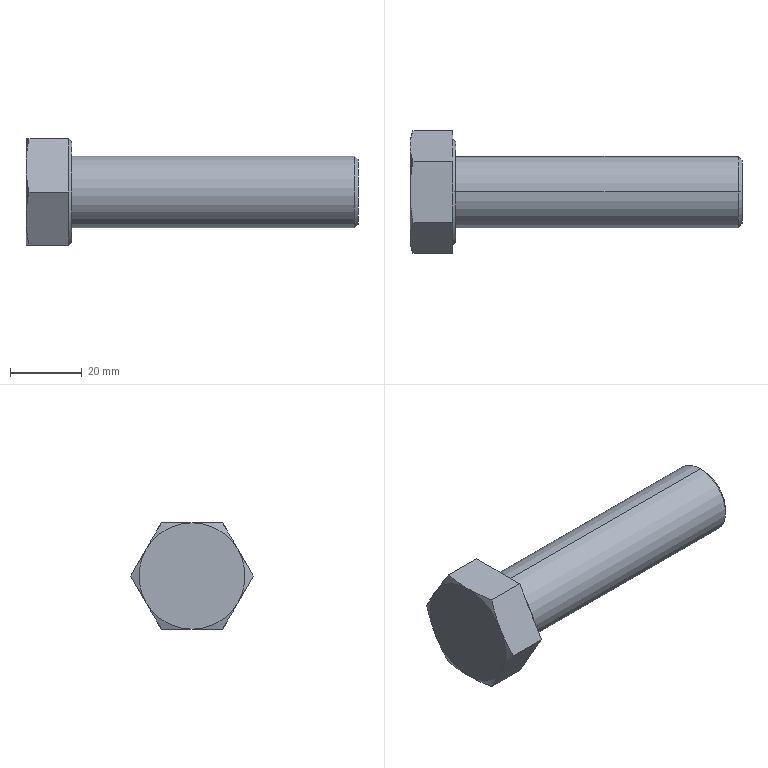Part | SolidWorks | features RevCut 3, Boss 1, Chamfer 1, Extrusion 1, Fillet 1, LPattern 1 | 1 solid | 27 faces | box 92.715 x 34.26 x 29.67 mm | volume 34696 mm3 | plane 15 | cone 10 | cylinder 2 | commonest cylinder face diameters 20 x2
STEP:
#1=CARTESIAN_POINT('',(92.715,0.,-9.));
#2=VERTEX_POINT('',#1);
#3=CARTESIAN_POINT('',(92.715,0.,9.));
#4=VERTEX_POINT('',#3);
#5=CARTESIAN_POINT('',(92.715,0.,0.));
#6=DIRECTION('',(1.,0.,0.));
#7=DIRECTION('',(0.,0.,-1.));
#8=AXIS2_PLACEMENT_3D('',#5,#6,#7);
#9=CIRCLE('',#8,9.);
#10=EDGE_CURVE('',#2,#4,#9,.T.);
#11=ORIENTED_EDGE('',*,*,#10,.F.);
#12=CARTESIAN_POINT('',(91.715,0.,-10.));
#13=VERTEX_POINT('',#12);
#14=CARTESIAN_POINT('',(92.715,0.,-9.));
#15=DIRECTION('',(-0.7071,0.,-0.7071));
#16=VECTOR('',#15,1000.);
#17=LINE('',#14,#16);
#18=EDGE_CURVE('',#2,#13,#17,.T.);
#19=ORIENTED_EDGE('',*,*,#18,.T.);
#20=CARTESIAN_POINT('',(91.715,0.,10.));
#21=VERTEX_POINT('',#20);
#22=CARTESIAN_POINT('',(91.715,0.,0.));
#23=DIRECTION('',(-1.,0.,0.));
#24=DIRECTION('',(0.,0.,-1.));
#25=AXIS2_PLACEMENT_3D('',#22,#23,#24);
#26=CIRCLE('',#25,10.);
#27=EDGE_CURVE('',#21,#13,#26,.T.);
#28=ORIENTED_EDGE('',*,*,#27,.F.);
#29=CARTESIAN_POINT('',(92.715,0.,9.));
#30=DIRECTION('',(-0.7071,0.,0.7071));
#31=VECTOR('',#30,1000.);
#32=LINE('',#29,#31);
#33=EDGE_CURVE('',#4,#21,#32,.T.);
#34=ORIENTED_EDGE('',*,*,#33,.F.);
#35=EDGE_LOOP('',(#11,#19,#28,#34));
#36=FACE_OUTER_BOUND('',#35,.T.);
#37=CARTESIAN_POINT('',(92.715,0.,0.));
#38=DIRECTION('',(-1.,0.,0.));
#39=DIRECTION('',(0.,0.,1.));
#40=AXIS2_PLACEMENT_3D('',#37,#38,#39);
#41=CONICAL_SURFACE('',#40,9.,0.7854);
#42=ADVANCED_FACE('',(#36),#41,.T.);
#43=ORIENTED_EDGE('',*,*,#27,.T.);
#44=CARTESIAN_POINT('',(12.715,0.,-10.));
#45=VERTEX_POINT('',#44);
#46=CARTESIAN_POINT('',(92.715,0.,-10.));
#47=DIRECTION('',(-1.,0.,0.));
#48=VECTOR('',#47,1000.);
#49=LINE('',#46,#48);
#50=EDGE_CURVE('',#13,#45,#49,.T.);
#51=ORIENTED_EDGE('',*,*,#50,.T.);
#52=CARTESIAN_POINT('',(12.715,0.,10.));
#53=VERTEX_POINT('',#52);
#54=CARTESIAN_POINT('',(12.715,0.,0.));
#55=DIRECTION('',(1.,0.,0.));
#56=DIRECTION('',(0.,0.,-1.));
#57=AXIS2_PLACEMENT_3D('',#54,#55,#56);
#58=CIRCLE('',#57,10.);
#59=EDGE_CURVE('',#45,#53,#58,.T.);
#60=ORIENTED_EDGE('',*,*,#59,.T.);
#61=CARTESIAN_POINT('',(92.715,0.,10.));
#62=DIRECTION('',(-1.,0.,0.));
#63=VECTOR('',#62,1000.);
#64=LINE('',#61,#63);
#65=EDGE_CURVE('',#21,#53,#64,.T.);
#66=ORIENTED_EDGE('',*,*,#65,.F.);
#67=EDGE_LOOP('',(#43,#51,#60,#66));
#68=FACE_OUTER_BOUND('',#67,.T.);
#69=CARTESIAN_POINT('',(92.715,0.,0.));
#70=DIRECTION('',(-1.,0.,0.));
#71=DIRECTION('',(0.,0.,1.));
#72=AXIS2_PLACEMENT_3D('',#69,#70,#71);
#73=CYLINDRICAL_SURFACE('',#72,10.);
#74=ADVANCED_FACE('',(#68),#73,.T.);
#75=CARTESIAN_POINT('',(12.715,0.,14.095));
#76=VERTEX_POINT('',#75);
#77=CARTESIAN_POINT('',(12.715,0.,-14.095));
#78=VERTEX_POINT('',#77);
#79=CARTESIAN_POINT('',(12.715,0.,0.));
#80=DIRECTION('',(-1.,0.,0.));
#81=DIRECTION('',(0.,0.,1.));
#82=AXIS2_PLACEMENT_3D('',#79,#80,#81);
#83=CIRCLE('',#82,14.095);
#84=EDGE_CURVE('',#76,#78,#83,.T.);
#85=ORIENTED_EDGE('',*,*,#84,.T.);
#86=CARTESIAN_POINT('',(11.975,0.,-14.835));
#87=VERTEX_POINT('',#86);
#88=CARTESIAN_POINT('',(11.915,0.,-14.895));
#89=DIRECTION('',(-0.7071,0.,-0.7071));
#90=VECTOR('',#89,1000.);
#91=LINE('',#88,#90);
#92=EDGE_CURVE('',#78,#87,#91,.T.);
#93=ORIENTED_EDGE('',*,*,#92,.T.);
#94=CARTESIAN_POINT('',(11.915,1.336,-14.835));
#95=VERTEX_POINT('',#94);
#96=CARTESIAN_POINT('',(11.975,0.,-14.835));
#97=CARTESIAN_POINT('',(11.975,0.4454,-14.835));
#98=CARTESIAN_POINT('',(11.955,0.8906,-14.835));
#99=CARTESIAN_POINT('',(11.915,1.336,-14.835));
#100=B_SPLINE_CURVE_WITH_KNOTS('',3,(#96,#97,#98,#99),.UNSPECIFIED.,.F.,.F.,(4,4),(0.008338,0.009669),.UNSPECIFIED.);
#101=EDGE_CURVE('',#87,#95,#100,.T.);
#102=ORIENTED_EDGE('',*,*,#101,.T.);
#103=CARTESIAN_POINT('',(11.915,12.18,-8.574));
#104=VERTEX_POINT('',#103);
#105=CARTESIAN_POINT('',(11.915,0.,0.));
#106=DIRECTION('',(-1.,0.,0.));
#107=DIRECTION('',(0.,0.,1.));
#108=AXIS2_PLACEMENT_3D('',#105,#106,#107);
#109=CIRCLE('',#108,14.895);
#110=EDGE_CURVE('',#104,#95,#109,.T.);
#111=ORIENTED_EDGE('',*,*,#110,.F.);
#112=CARTESIAN_POINT('',(11.915,13.515,-6.261));
#113=VERTEX_POINT('',#112);
#114=CARTESIAN_POINT('',(11.915,12.18,-8.574));
#115=CARTESIAN_POINT('',(11.995,12.625,-7.803));
#116=CARTESIAN_POINT('',(11.995,13.07,-7.032));
#117=CARTESIAN_POINT('',(11.915,13.515,-6.261));
#118=B_SPLINE_CURVE_WITH_KNOTS('',3,(#114,#115,#116,#117),.UNSPECIFIED.,.F.,.F.,(4,4),(0.000002229,0.002673),.UNSPECIFIED.);
#119=EDGE_CURVE('',#104,#113,#118,.T.);
#120=ORIENTED_EDGE('',*,*,#119,.T.);
#121=CARTESIAN_POINT('',(11.915,13.515,6.261));
#122=VERTEX_POINT('',#121);
#123=CARTESIAN_POINT('',(11.915,0.,0.));
#124=DIRECTION('',(-1.,0.,0.));
#125=DIRECTION('',(0.,0.,1.));
#126=AXIS2_PLACEMENT_3D('',#123,#124,#125);
#127=CIRCLE('',#126,14.895);
#128=EDGE_CURVE('',#122,#113,#127,.T.);
#129=ORIENTED_EDGE('',*,*,#128,.F.);
#130=CARTESIAN_POINT('',(11.915,12.18,8.574));
#131=VERTEX_POINT('',#130);
#132=CARTESIAN_POINT('',(11.915,13.515,6.261));
#133=CARTESIAN_POINT('',(11.995,13.07,7.032));
#134=CARTESIAN_POINT('',(11.995,12.625,7.803));
#135=CARTESIAN_POINT('',(11.915,12.18,8.574));
#136=B_SPLINE_CURVE_WITH_KNOTS('',3,(#132,#133,#134,#135),.UNSPECIFIED.,.F.,.F.,(4,4),(0.000002229,0.002673),.UNSPECIFIED.);
#137=EDGE_CURVE('',#122,#131,#136,.T.);
#138=ORIENTED_EDGE('',*,*,#137,.T.);
#139=CARTESIAN_POINT('',(11.915,1.336,14.835));
#140=VERTEX_POINT('',#139);
#141=CARTESIAN_POINT('',(11.915,0.,0.));
#142=DIRECTION('',(-1.,0.,0.));
#143=DIRECTION('',(0.,0.,1.));
#144=AXIS2_PLACEMENT_3D('',#141,#142,#143);
#145=CIRCLE('',#144,14.895);
#146=EDGE_CURVE('',#140,#131,#145,.T.);
#147=ORIENTED_EDGE('',*,*,#146,.F.);
#148=CARTESIAN_POINT('',(11.975,0.,14.835));
#149=VERTEX_POINT('',#148);
#150=CARTESIAN_POINT('',(11.915,1.336,14.835));
#151=CARTESIAN_POINT('',(11.955,0.8906,14.835));
#152=CARTESIAN_POINT('',(11.975,0.4454,14.835));
#153=CARTESIAN_POINT('',(11.975,0.,14.835));
#154=B_SPLINE_CURVE_WITH_KNOTS('',3,(#150,#151,#152,#153),.UNSPECIFIED.,.F.,.F.,(4,4),(0.007682,0.009012),.UNSPECIFIED.);
#155=EDGE_CURVE('',#140,#149,#154,.T.);
#156=ORIENTED_EDGE('',*,*,#155,.T.);
#157=CARTESIAN_POINT('',(11.915,0.,14.895));
#158=DIRECTION('',(-0.7071,0.,0.7071));
#159=VECTOR('',#158,1000.);
#160=LINE('',#157,#159);
#161=EDGE_CURVE('',#76,#149,#160,.T.);
#162=ORIENTED_EDGE('',*,*,#161,.F.);
#163=EDGE_LOOP('',(#85,#93,#102,#111,#120,#129,#138,#147,#156,#162));
#164=FACE_OUTER_BOUND('',#163,.T.);
#165=CARTESIAN_POINT('',(11.915,0.,0.));
#166=DIRECTION('',(-1.,0.,0.));
#167=DIRECTION('',(0.,0.,1.));
#168=AXIS2_PLACEMENT_3D('',#165,#166,#167);
#169=CONICAL_SURFACE('',#168,14.895,0.7854);
#170=ADVANCED_FACE('',(#164),#169,.T.);
#171=ORIENTED_EDGE('',*,*,#84,.F.);
#172=CARTESIAN_POINT('',(12.715,0.,0.));
#173=DIRECTION('',(-1.,0.,0.));
#174=DIRECTION('',(0.,0.,1.));
#175=AXIS2_PLACEMENT_3D('',#172,#173,#174);
#176=CIRCLE('',#175,14.095);
#177=EDGE_CURVE('',#78,#76,#176,.T.);
#178=ORIENTED_EDGE('',*,*,#177,.F.);
#179=EDGE_LOOP('',(#171,#178));
#180=FACE_OUTER_BOUND('',#179,.T.);
#181=CARTESIAN_POINT('',(12.715,0.,0.));
#182=DIRECTION('',(1.,0.,0.));
#183=DIRECTION('',(0.,0.,-1.));
#184=AXIS2_PLACEMENT_3D('',#181,#182,#183);
#185=CIRCLE('',#184,10.);
#186=EDGE_CURVE('',#53,#45,#185,.T.);
#187=ORIENTED_EDGE('',*,*,#186,.F.);
#188=ORIENTED_EDGE('',*,*,#59,.F.);
#189=EDGE_LOOP('',(#187,#188));
#190=FACE_BOUND('',#189,.T.);
#191=CARTESIAN_POINT('',(12.715,-8.565,-14.835));
#192=DIRECTION('',(1.,0.,0.));
#193=DIRECTION('',(0.,0.,-1.));
#194=AXIS2_PLACEMENT_3D('',#191,#192,#193);
#195=PLANE('',#194);
#196=ADVANCED_FACE('',(#180,#190),#195,.T.);
#197=CARTESIAN_POINT('',(0.8353,-8.565,-14.835));
#198=VERTEX_POINT('',#197);
#199=CARTESIAN_POINT('',(0.,-12.847,-7.417));
#200=VERTEX_POINT('',#199);
#201=CARTESIAN_POINT('',(0.8353,-8.565,-14.835));
#202=CARTESIAN_POINT('',(0.5755,-9.279,-13.599));
#203=CARTESIAN_POINT('',(0.3646,-9.992,-12.363));
#204=CARTESIAN_POINT('',(0.07638,-11.42,-9.89));
#205=CARTESIAN_POINT('',(0.,-12.134,-8.654));
#206=CARTESIAN_POINT('',(0.,-12.847,-7.417));
#207=B_SPLINE_CURVE_WITH_KNOTS('',3,(#201,#202,#203,#204,#205,#206),.UNSPECIFIED.,.F.,.F.,(4,2,4),(0.000000231,0.004283,0.008565),.UNSPECIFIED.);
#208=EDGE_CURVE('',#198,#200,#207,.T.);
#209=ORIENTED_EDGE('',*,*,#208,.F.);
#210=CARTESIAN_POINT('',(11.915,-8.565,-14.835));
#211=VERTEX_POINT('',#210);
#212=CARTESIAN_POINT('',(12.715,-8.565,-14.835));
#213=DIRECTION('',(-1.,0.,0.));
#214=VECTOR('',#213,1000.);
#215=LINE('',#212,#214);
#216=EDGE_CURVE('',#211,#198,#215,.T.);
#217=ORIENTED_EDGE('',*,*,#216,.F.);
#218=CARTESIAN_POINT('',(11.915,-12.18,-8.574));
#219=VERTEX_POINT('',#218);
#220=CARTESIAN_POINT('',(11.915,-17.13,0.));
#221=DIRECTION('',(0.,0.5,-0.866));
#222=VECTOR('',#221,1000.);
#223=LINE('',#220,#222);
#224=EDGE_CURVE('',#219,#211,#223,.T.);
#225=ORIENTED_EDGE('',*,*,#224,.F.);
#226=CARTESIAN_POINT('',(11.915,-13.515,-6.261));
#227=VERTEX_POINT('',#226);
#228=CARTESIAN_POINT('',(11.915,-13.515,-6.261));
#229=CARTESIAN_POINT('',(11.995,-13.07,-7.032));
#230=CARTESIAN_POINT('',(11.995,-12.625,-7.803));
#231=CARTESIAN_POINT('',(11.915,-12.18,-8.574));
#232=B_SPLINE_CURVE_WITH_KNOTS('',3,(#228,#229,#230,#231),.UNSPECIFIED.,.F.,.F.,(4,4),(0.000002229,0.002673),.UNSPECIFIED.);
#233=EDGE_CURVE('',#227,#219,#232,.T.);
#234=ORIENTED_EDGE('',*,*,#233,.F.);
#235=CARTESIAN_POINT('',(11.915,-17.13,0.));
#236=VERTEX_POINT('',#235);
#237=CARTESIAN_POINT('',(11.915,-17.13,0.));
#238=DIRECTION('',(0.,0.5,-0.866));
#239=VECTOR('',#238,1000.);
#240=LINE('',#237,#239);
#241=EDGE_CURVE('',#236,#227,#240,.T.);
#242=ORIENTED_EDGE('',*,*,#241,.F.);
#243=CARTESIAN_POINT('',(0.8353,-17.13,0.));
#244=VERTEX_POINT('',#243);
#245=CARTESIAN_POINT('',(12.715,-17.13,0.));
#246=DIRECTION('',(-1.,0.,0.));
#247=VECTOR('',#246,1000.);
#248=LINE('',#245,#247);
#249=EDGE_CURVE('',#236,#244,#248,.T.);
#250=ORIENTED_EDGE('',*,*,#249,.T.);
#251=CARTESIAN_POINT('',(0.,-12.847,-7.417));
#252=CARTESIAN_POINT('',(0.,-13.561,-6.181));
#253=CARTESIAN_POINT('',(0.07638,-14.275,-4.945));
#254=CARTESIAN_POINT('',(0.3646,-15.702,-2.472));
#255=CARTESIAN_POINT('',(0.5755,-16.416,-1.236));
#256=CARTESIAN_POINT('',(0.8353,-17.13,0.));
#257=B_SPLINE_CURVE_WITH_KNOTS('',3,(#251,#252,#253,#254,#255,#256),.UNSPECIFIED.,.F.,.F.,(4,2,4),(0.008565,0.01285,0.01713),.UNSPECIFIED.);
#258=EDGE_CURVE('',#200,#244,#257,.T.);
#259=ORIENTED_EDGE('',*,*,#258,.F.);
#260=EDGE_LOOP('',(#209,#217,#225,#234,#242,#250,#259));
#261=FACE_OUTER_BOUND('',#260,.T.);
#262=CARTESIAN_POINT('',(12.715,-17.13,0.));
#263=DIRECTION('',(0.,0.866,0.5));
#264=DIRECTION('',(0.,-0.5,0.866));
#265=AXIS2_PLACEMENT_3D('',#262,#263,#264);
#266=PLANE('',#265);
#267=ADVANCED_FACE('',(#261),#266,.F.);
#268=CARTESIAN_POINT('',(0.8353,8.565,-14.835));
#269=VERTEX_POINT('',#268);
#270=CARTESIAN_POINT('',(0.,0.,-14.835));
#271=VERTEX_POINT('',#270);
#272=CARTESIAN_POINT('',(0.8353,8.565,-14.835));
#273=CARTESIAN_POINT('',(0.5762,7.141,-14.835));
#274=CARTESIAN_POINT('',(0.3651,5.714,-14.835));
#275=CARTESIAN_POINT('',(0.07668,2.859,-14.835));
#276=CARTESIAN_POINT('',(0.,1.43,-14.835));
#277=CARTESIAN_POINT('',(0.,0.,-14.835));
#278=B_SPLINE_CURVE_WITH_KNOTS('',3,(#272,#273,#274,#275,#276,#277),.UNSPECIFIED.,.F.,.F.,(4,2,4),(0.03088,0.0352,0.03952),.UNSPECIFIED.);
#279=EDGE_CURVE('',#269,#271,#278,.T.);
#280=ORIENTED_EDGE('',*,*,#279,.F.);
#281=CARTESIAN_POINT('',(11.915,8.565,-14.835));
#282=VERTEX_POINT('',#281);
#283=CARTESIAN_POINT('',(12.715,8.565,-14.835));
#284=DIRECTION('',(-1.,0.,0.));
#285=VECTOR('',#284,1000.);
#286=LINE('',#283,#285);
#287=EDGE_CURVE('',#282,#269,#286,.T.);
#288=ORIENTED_EDGE('',*,*,#287,.F.);
#289=CARTESIAN_POINT('',(11.915,-8.565,-14.835));
#290=DIRECTION('',(0.,1.,0.));
#291=VECTOR('',#290,1000.);
#292=LINE('',#289,#291);
#293=EDGE_CURVE('',#95,#282,#292,.T.);
#294=ORIENTED_EDGE('',*,*,#293,.F.);
#295=ORIENTED_EDGE('',*,*,#101,.F.);
#296=CARTESIAN_POINT('',(11.915,-1.336,-14.835));
#297=VERTEX_POINT('',#296);
#298=CARTESIAN_POINT('',(11.915,-1.336,-14.835));
#299=CARTESIAN_POINT('',(11.955,-0.8902,-14.835));
#300=CARTESIAN_POINT('',(11.975,-0.445,-14.835));
#301=CARTESIAN_POINT('',(11.975,0.,-14.835));
#302=B_SPLINE_CURVE_WITH_KNOTS('',3,(#298,#299,#300,#301),.UNSPECIFIED.,.F.,.F.,(4,4),(0.007008,0.008338),.UNSPECIFIED.);
#303=EDGE_CURVE('',#297,#87,#302,.T.);
#304=ORIENTED_EDGE('',*,*,#303,.F.);
#305=CARTESIAN_POINT('',(11.915,-8.565,-14.835));
#306=DIRECTION('',(0.,1.,0.));
#307=VECTOR('',#306,1000.);
#308=LINE('',#305,#307);
#309=EDGE_CURVE('',#211,#297,#308,.T.);
#310=ORIENTED_EDGE('',*,*,#309,.F.);
#311=ORIENTED_EDGE('',*,*,#216,.T.);
#312=CARTESIAN_POINT('',(0.,0.,-14.835));
#313=CARTESIAN_POINT('',(0.,-1.426,-14.835));
#314=CARTESIAN_POINT('',(0.07627,-2.854,-14.835));
#315=CARTESIAN_POINT('',(0.3649,-5.713,-14.835));
#316=CARTESIAN_POINT('',(0.5772,-7.147,-14.835));
#317=CARTESIAN_POINT('',(0.8353,-8.565,-14.835));
#318=B_SPLINE_CURVE_WITH_KNOTS('',3,(#312,#313,#314,#315,#316,#317),.UNSPECIFIED.,.F.,.F.,(4,2,4),(0.03952,0.04383,0.04813),.UNSPECIFIED.);
#319=EDGE_CURVE('',#271,#198,#318,.T.);
#320=ORIENTED_EDGE('',*,*,#319,.F.);
#321=EDGE_LOOP('',(#280,#288,#294,#295,#304,#310,#311,#320));
#322=FACE_OUTER_BOUND('',#321,.T.);
#323=CARTESIAN_POINT('',(12.715,-8.565,-14.835));
#324=DIRECTION('',(0.,0.,1.));
#325=DIRECTION('',(1.,0.,0.));
#326=AXIS2_PLACEMENT_3D('',#323,#324,#325);
#327=PLANE('',#326);
#328=ADVANCED_FACE('',(#322),#327,.F.);
#329=CARTESIAN_POINT('',(0.8353,17.13,0.));
#330=VERTEX_POINT('',#329);
#331=CARTESIAN_POINT('',(0.,12.847,-7.418));
#332=VERTEX_POINT('',#331);
#333=CARTESIAN_POINT('',(0.8353,17.13,0.));
#334=CARTESIAN_POINT('',(0.5755,16.416,-1.236));
#335=CARTESIAN_POINT('',(0.3646,15.702,-2.472));
#336=CARTESIAN_POINT('',(0.07638,14.275,-4.945));
#337=CARTESIAN_POINT('',(0.,13.561,-6.181));
#338=CARTESIAN_POINT('',(0.,12.847,-7.418));
#339=B_SPLINE_CURVE_WITH_KNOTS('',3,(#333,#334,#335,#336,#337,#338),.UNSPECIFIED.,.F.,.F.,(4,2,4),(0.000000231,0.004283,0.008565),.UNSPECIFIED.);
#340=EDGE_CURVE('',#330,#332,#339,.T.);
#341=ORIENTED_EDGE('',*,*,#340,.F.);
#342=CARTESIAN_POINT('',(11.915,17.13,0.));
#343=VERTEX_POINT('',#342);
#344=CARTESIAN_POINT('',(12.715,17.13,0.));
#345=DIRECTION('',(-1.,0.,0.));
#346=VECTOR('',#345,1000.);
#347=LINE('',#344,#346);
#348=EDGE_CURVE('',#343,#330,#347,.T.);
#349=ORIENTED_EDGE('',*,*,#348,.F.);
#350=CARTESIAN_POINT('',(11.915,8.565,-14.835));
#351=DIRECTION('',(0.,0.5,0.866));
#352=VECTOR('',#351,1000.);
#353=LINE('',#350,#352);
#354=EDGE_CURVE('',#113,#343,#353,.T.);
#355=ORIENTED_EDGE('',*,*,#354,.F.);
#356=ORIENTED_EDGE('',*,*,#119,.F.);
#357=CARTESIAN_POINT('',(11.915,8.565,-14.835));
#358=DIRECTION('',(0.,0.5,0.866));
#359=VECTOR('',#358,1000.);
#360=LINE('',#357,#359);
#361=EDGE_CURVE('',#282,#104,#360,.T.);
#362=ORIENTED_EDGE('',*,*,#361,.F.);
#363=ORIENTED_EDGE('',*,*,#287,.T.);
#364=CARTESIAN_POINT('',(0.,12.847,-7.418));
#365=CARTESIAN_POINT('',(0.,12.134,-8.654));
#366=CARTESIAN_POINT('',(0.07638,11.42,-9.89));
#367=CARTESIAN_POINT('',(0.3646,9.992,-12.362));
#368=CARTESIAN_POINT('',(0.5755,9.279,-13.599));
#369=CARTESIAN_POINT('',(0.8353,8.565,-14.835));
#370=B_SPLINE_CURVE_WITH_KNOTS('',3,(#364,#365,#366,#367,#368,#369),.UNSPECIFIED.,.F.,.F.,(4,2,4),(0.008565,0.01285,0.01713),.UNSPECIFIED.);
#371=EDGE_CURVE('',#332,#269,#370,.T.);
#372=ORIENTED_EDGE('',*,*,#371,.F.);
#373=EDGE_LOOP('',(#341,#349,#355,#356,#362,#363,#372));
#374=FACE_OUTER_BOUND('',#373,.T.);
#375=CARTESIAN_POINT('',(12.715,8.565,-14.835));
#376=DIRECTION('',(0.,-0.866,0.5));
#377=DIRECTION('',(0.,-0.5,-0.866));
#378=AXIS2_PLACEMENT_3D('',#375,#376,#377);
#379=PLANE('',#378);
#380=ADVANCED_FACE('',(#374),#379,.F.);
#381=CARTESIAN_POINT('',(0.8353,8.565,14.835));
#382=VERTEX_POINT('',#381);
#383=CARTESIAN_POINT('',(0.,12.847,7.417));
#384=VERTEX_POINT('',#383);
#385=CARTESIAN_POINT('',(0.8353,8.565,14.835));
#386=CARTESIAN_POINT('',(0.5755,9.279,13.599));
#387=CARTESIAN_POINT('',(0.3646,9.992,12.363));
#388=CARTESIAN_POINT('',(0.07638,11.42,9.89));
#389=CARTESIAN_POINT('',(0.,12.134,8.654));
#390=CARTESIAN_POINT('',(0.,12.847,7.417));
#391=B_SPLINE_CURVE_WITH_KNOTS('',3,(#385,#386,#387,#388,#389,#390),.UNSPECIFIED.,.F.,.F.,(4,2,4),(0.000000231,0.004283,0.008565),.UNSPECIFIED.);
#392=EDGE_CURVE('',#382,#384,#391,.T.);
#393=ORIENTED_EDGE('',*,*,#392,.F.);
#394=CARTESIAN_POINT('',(11.915,8.565,14.835));
#395=VERTEX_POINT('',#394);
#396=CARTESIAN_POINT('',(12.715,8.565,14.835));
#397=DIRECTION('',(-1.,0.,0.));
#398=VECTOR('',#397,1000.);
#399=LINE('',#396,#398);
#400=EDGE_CURVE('',#395,#382,#399,.T.);
#401=ORIENTED_EDGE('',*,*,#400,.F.);
#402=CARTESIAN_POINT('',(11.915,17.13,0.));
#403=DIRECTION('',(0.,-0.5,0.866));
#404=VECTOR('',#403,1000.);
#405=LINE('',#402,#404);
#406=EDGE_CURVE('',#131,#395,#405,.T.);
#407=ORIENTED_EDGE('',*,*,#406,.F.);
#408=ORIENTED_EDGE('',*,*,#137,.F.);
#409=CARTESIAN_POINT('',(11.915,17.13,0.));
#410=DIRECTION('',(0.,-0.5,0.866));
#411=VECTOR('',#410,1000.);
#412=LINE('',#409,#411);
#413=EDGE_CURVE('',#343,#122,#412,.T.);
#414=ORIENTED_EDGE('',*,*,#413,.F.);
#415=ORIENTED_EDGE('',*,*,#348,.T.);
#416=CARTESIAN_POINT('',(0.,12.847,7.417));
#417=CARTESIAN_POINT('',(0.,13.561,6.181));
#418=CARTESIAN_POINT('',(0.07638,14.275,4.945));
#419=CARTESIAN_POINT('',(0.3646,15.702,2.473));
#420=CARTESIAN_POINT('',(0.5755,16.416,1.236));
#421=CARTESIAN_POINT('',(0.8353,17.13,0.));
#422=B_SPLINE_CURVE_WITH_KNOTS('',3,(#416,#417,#418,#419,#420,#421),.UNSPECIFIED.,.F.,.F.,(4,2,4),(0.008565,0.01285,0.01713),.UNSPECIFIED.);
#423=EDGE_CURVE('',#384,#330,#422,.T.);
#424=ORIENTED_EDGE('',*,*,#423,.F.);
#425=EDGE_LOOP('',(#393,#401,#407,#408,#414,#415,#424));
#426=FACE_OUTER_BOUND('',#425,.T.);
#427=CARTESIAN_POINT('',(12.715,17.13,0.));
#428=DIRECTION('',(0.,-0.866,-0.5));
#429=DIRECTION('',(0.,0.5,-0.866));
#430=AXIS2_PLACEMENT_3D('',#427,#428,#429);
#431=PLANE('',#430);
#432=ADVANCED_FACE('',(#426),#431,.F.);
#433=CARTESIAN_POINT('',(0.8353,-8.565,14.835));
#434=VERTEX_POINT('',#433);
#435=CARTESIAN_POINT('',(0.,0.,14.835));
#436=VERTEX_POINT('',#435);
#437=CARTESIAN_POINT('',(0.8353,-8.565,14.835));
#438=CARTESIAN_POINT('',(0.5772,-7.147,14.835));
#439=CARTESIAN_POINT('',(0.3649,-5.713,14.835));
#440=CARTESIAN_POINT('',(0.07627,-2.854,14.835));
#441=CARTESIAN_POINT('',(0.,-1.426,14.835));
#442=CARTESIAN_POINT('',(0.,0.,14.835));
#443=B_SPLINE_CURVE_WITH_KNOTS('',3,(#437,#438,#439,#440,#441,#442),.UNSPECIFIED.,.F.,.F.,(4,2,4),(0.01457,0.01889,0.0232),.UNSPECIFIED.);
#444=EDGE_CURVE('',#434,#436,#443,.T.);
#445=ORIENTED_EDGE('',*,*,#444,.F.);
#446=CARTESIAN_POINT('',(11.915,-8.565,14.835));
#447=VERTEX_POINT('',#446);
#448=CARTESIAN_POINT('',(12.715,-8.565,14.835));
#449=DIRECTION('',(-1.,0.,0.));
#450=VECTOR('',#449,1000.);
#451=LINE('',#448,#450);
#452=EDGE_CURVE('',#447,#434,#451,.T.);
#453=ORIENTED_EDGE('',*,*,#452,.F.);
#454=CARTESIAN_POINT('',(11.915,-1.336,14.835));
#455=VERTEX_POINT('',#454);
#456=CARTESIAN_POINT('',(11.915,8.565,14.835));
#457=DIRECTION('',(0.,-1.,0.));
#458=VECTOR('',#457,1000.);
#459=LINE('',#456,#458);
#460=EDGE_CURVE('',#455,#447,#459,.T.);
#461=ORIENTED_EDGE('',*,*,#460,.F.);
#462=CARTESIAN_POINT('',(11.975,0.,14.835));
#463=CARTESIAN_POINT('',(11.975,-0.445,14.835));
#464=CARTESIAN_POINT('',(11.955,-0.8902,14.835));
#465=CARTESIAN_POINT('',(11.915,-1.336,14.835));
#466=B_SPLINE_CURVE_WITH_KNOTS('',3,(#462,#463,#464,#465),.UNSPECIFIED.,.F.,.F.,(4,4),(0.009012,0.01034),.UNSPECIFIED.);
#467=EDGE_CURVE('',#149,#455,#466,.T.);
#468=ORIENTED_EDGE('',*,*,#467,.F.);
#469=ORIENTED_EDGE('',*,*,#155,.F.);
#470=CARTESIAN_POINT('',(11.915,8.565,14.835));
#471=DIRECTION('',(0.,-1.,0.));
#472=VECTOR('',#471,1000.);
#473=LINE('',#470,#472);
#474=EDGE_CURVE('',#395,#140,#473,.T.);
#475=ORIENTED_EDGE('',*,*,#474,.F.);
#476=ORIENTED_EDGE('',*,*,#400,.T.);
#477=CARTESIAN_POINT('',(0.,0.,14.835));
#478=CARTESIAN_POINT('',(0.,1.43,14.835));
#479=CARTESIAN_POINT('',(0.07668,2.859,14.835));
#480=CARTESIAN_POINT('',(0.3651,5.714,14.835));
#481=CARTESIAN_POINT('',(0.5762,7.141,14.835));
#482=CARTESIAN_POINT('',(0.8353,8.565,14.835));
#483=B_SPLINE_CURVE_WITH_KNOTS('',3,(#477,#478,#479,#480,#481,#482),.UNSPECIFIED.,.F.,.F.,(4,2,4),(0.0232,0.02753,0.03186),.UNSPECIFIED.);
#484=EDGE_CURVE('',#436,#382,#483,.T.);
#485=ORIENTED_EDGE('',*,*,#484,.F.);
#486=EDGE_LOOP('',(#445,#453,#461,#468,#469,#475,#476,#485));
#487=FACE_OUTER_BOUND('',#486,.T.);
#488=CARTESIAN_POINT('',(12.715,8.565,14.835));
#489=DIRECTION('',(0.,0.,-1.));
#490=DIRECTION('',(0.,1.,0.));
#491=AXIS2_PLACEMENT_3D('',#488,#489,#490);
#492=PLANE('',#491);
#493=ADVANCED_FACE('',(#487),#492,.F.);
#494=CARTESIAN_POINT('',(0.,-12.847,7.418));
#495=VERTEX_POINT('',#494);
#496=CARTESIAN_POINT('',(0.8353,-17.13,0.));
#497=CARTESIAN_POINT('',(0.5755,-16.416,1.236));
#498=CARTESIAN_POINT('',(0.3646,-15.702,2.473));
#499=CARTESIAN_POINT('',(0.07638,-14.275,4.945));
#500=CARTESIAN_POINT('',(0.,-13.561,6.181));
#501=CARTESIAN_POINT('',(0.,-12.847,7.418));
#502=B_SPLINE_CURVE_WITH_KNOTS('',3,(#496,#497,#498,#499,#500,#501),.UNSPECIFIED.,.F.,.F.,(4,2,4),(0.000000231,0.004283,0.008565),.UNSPECIFIED.);
#503=EDGE_CURVE('',#244,#495,#502,.T.);
#504=ORIENTED_EDGE('',*,*,#503,.F.);
#505=ORIENTED_EDGE('',*,*,#249,.F.);
#506=CARTESIAN_POINT('',(11.915,-13.515,6.261));
#507=VERTEX_POINT('',#506);
#508=CARTESIAN_POINT('',(11.915,-8.565,14.835));
#509=DIRECTION('',(0.,-0.5,-0.866));
#510=VECTOR('',#509,1000.);
#511=LINE('',#508,#510);
#512=EDGE_CURVE('',#507,#236,#511,.T.);
#513=ORIENTED_EDGE('',*,*,#512,.F.);
#514=CARTESIAN_POINT('',(11.915,-12.18,8.574));
#515=VERTEX_POINT('',#514);
#516=CARTESIAN_POINT('',(11.915,-12.18,8.574));
#517=CARTESIAN_POINT('',(11.995,-12.625,7.803));
#518=CARTESIAN_POINT('',(11.995,-13.07,7.032));
#519=CARTESIAN_POINT('',(11.915,-13.515,6.261));
#520=B_SPLINE_CURVE_WITH_KNOTS('',3,(#516,#517,#518,#519),.UNSPECIFIED.,.F.,.F.,(4,4),(0.000002229,0.002673),.UNSPECIFIED.);
#521=EDGE_CURVE('',#515,#507,#520,.T.);
#522=ORIENTED_EDGE('',*,*,#521,.F.);
#523=CARTESIAN_POINT('',(11.915,-8.565,14.835));
#524=DIRECTION('',(0.,-0.5,-0.866));
#525=VECTOR('',#524,1000.);
#526=LINE('',#523,#525);
#527=EDGE_CURVE('',#447,#515,#526,.T.);
#528=ORIENTED_EDGE('',*,*,#527,.F.);
#529=ORIENTED_EDGE('',*,*,#452,.T.);
#530=CARTESIAN_POINT('',(0.,-12.847,7.418));
#531=CARTESIAN_POINT('',(0.,-12.134,8.654));
#532=CARTESIAN_POINT('',(0.07638,-11.42,9.89));
#533=CARTESIAN_POINT('',(0.3646,-9.992,12.363));
#534=CARTESIAN_POINT('',(0.5755,-9.279,13.599));
#535=CARTESIAN_POINT('',(0.8353,-8.565,14.835));
#536=B_SPLINE_CURVE_WITH_KNOTS('',3,(#530,#531,#532,#533,#534,#535),.UNSPECIFIED.,.F.,.F.,(4,2,4),(0.008565,0.01285,0.01713),.UNSPECIFIED.);
#537=EDGE_CURVE('',#495,#434,#536,.T.);
#538=ORIENTED_EDGE('',*,*,#537,.F.);
#539=EDGE_LOOP('',(#504,#505,#513,#522,#528,#529,#538));
#540=FACE_OUTER_BOUND('',#539,.T.);
#541=CARTESIAN_POINT('',(12.715,-8.565,14.835));
#542=DIRECTION('',(0.,0.866,-0.5));
#543=DIRECTION('',(0.,0.5,0.866));
#544=AXIS2_PLACEMENT_3D('',#541,#542,#543);
#545=PLANE('',#544);
#546=ADVANCED_FACE('',(#540),#545,.F.);
#547=ORIENTED_EDGE('',*,*,#224,.T.);
#548=ORIENTED_EDGE('',*,*,#309,.T.);
#549=CARTESIAN_POINT('',(11.915,0.,0.));
#550=DIRECTION('',(-1.,0.,0.));
#551=DIRECTION('',(0.,0.,1.));
#552=AXIS2_PLACEMENT_3D('',#549,#550,#551);
#553=CIRCLE('',#552,14.895);
#554=EDGE_CURVE('',#297,#219,#553,.T.);
#555=ORIENTED_EDGE('',*,*,#554,.T.);
#556=EDGE_LOOP('',(#547,#548,#555));
#557=FACE_OUTER_BOUND('',#556,.T.);
#558=CARTESIAN_POINT('',(11.915,14.895,0.));
#559=DIRECTION('',(1.,0.,0.));
#560=DIRECTION('',(0.,0.,-1.));
#561=AXIS2_PLACEMENT_3D('',#558,#559,#560);
#562=PLANE('',#561);
#563=ADVANCED_FACE('',(#557),#562,.T.);
#564=ORIENTED_EDGE('',*,*,#293,.T.);
#565=ORIENTED_EDGE('',*,*,#361,.T.);
#566=ORIENTED_EDGE('',*,*,#110,.T.);
#567=EDGE_LOOP('',(#564,#565,#566));
#568=FACE_OUTER_BOUND('',#567,.T.);
#569=CARTESIAN_POINT('',(11.915,14.895,0.));
#570=DIRECTION('',(1.,0.,0.));
#571=DIRECTION('',(0.,0.,-1.));
#572=AXIS2_PLACEMENT_3D('',#569,#570,#571);
#573=PLANE('',#572);
#574=ADVANCED_FACE('',(#568),#573,.T.);
#575=ORIENTED_EDGE('',*,*,#354,.T.);
#576=ORIENTED_EDGE('',*,*,#413,.T.);
#577=ORIENTED_EDGE('',*,*,#128,.T.);
#578=EDGE_LOOP('',(#575,#576,#577));
#579=FACE_OUTER_BOUND('',#578,.T.);
#580=CARTESIAN_POINT('',(11.915,14.895,0.));
#581=DIRECTION('',(1.,0.,0.));
#582=DIRECTION('',(0.,0.,-1.));
#583=AXIS2_PLACEMENT_3D('',#580,#581,#582);
#584=PLANE('',#583);
#585=ADVANCED_FACE('',(#579),#584,.T.);
#586=ORIENTED_EDGE('',*,*,#406,.T.);
#587=ORIENTED_EDGE('',*,*,#474,.T.);
#588=ORIENTED_EDGE('',*,*,#146,.T.);
#589=EDGE_LOOP('',(#586,#587,#588));
#590=FACE_OUTER_BOUND('',#589,.T.);
#591=CARTESIAN_POINT('',(11.915,14.895,0.));
#592=DIRECTION('',(1.,0.,0.));
#593=DIRECTION('',(0.,0.,-1.));
#594=AXIS2_PLACEMENT_3D('',#591,#592,#593);
#595=PLANE('',#594);
#596=ADVANCED_FACE('',(#590),#595,.T.);
#597=ORIENTED_EDGE('',*,*,#460,.T.);
#598=ORIENTED_EDGE('',*,*,#527,.T.);
#599=CARTESIAN_POINT('',(11.915,0.,0.));
#600=DIRECTION('',(-1.,0.,0.));
#601=DIRECTION('',(0.,0.,1.));
#602=AXIS2_PLACEMENT_3D('',#599,#600,#601);
#603=CIRCLE('',#602,14.895);
#604=EDGE_CURVE('',#515,#455,#603,.T.);
#605=ORIENTED_EDGE('',*,*,#604,.T.);
#606=EDGE_LOOP('',(#597,#598,#605));
#607=FACE_OUTER_BOUND('',#606,.T.);
#608=CARTESIAN_POINT('',(11.915,14.895,0.));
#609=DIRECTION('',(1.,0.,0.));
#610=DIRECTION('',(0.,0.,-1.));
#611=AXIS2_PLACEMENT_3D('',#608,#609,#610);
#612=PLANE('',#611);
#613=ADVANCED_FACE('',(#607),#612,.T.);
#614=ORIENTED_EDGE('',*,*,#241,.T.);
#615=CARTESIAN_POINT('',(11.915,0.,0.));
#616=DIRECTION('',(-1.,0.,0.));
#617=DIRECTION('',(0.,0.,1.));
#618=AXIS2_PLACEMENT_3D('',#615,#616,#617);
#619=CIRCLE('',#618,14.895);
#620=EDGE_CURVE('',#227,#507,#619,.T.);
#621=ORIENTED_EDGE('',*,*,#620,.T.);
#622=ORIENTED_EDGE('',*,*,#512,.T.);
#623=EDGE_LOOP('',(#614,#621,#622));
#624=FACE_OUTER_BOUND('',#623,.T.);
#625=CARTESIAN_POINT('',(11.915,14.895,0.));
#626=DIRECTION('',(1.,0.,0.));
#627=DIRECTION('',(0.,0.,-1.));
#628=AXIS2_PLACEMENT_3D('',#625,#626,#627);
#629=PLANE('',#628);
#630=ADVANCED_FACE('',(#624),#629,.T.);
#631=ORIENTED_EDGE('',*,*,#92,.F.);
#632=ORIENTED_EDGE('',*,*,#177,.T.);
#633=ORIENTED_EDGE('',*,*,#161,.T.);
#634=ORIENTED_EDGE('',*,*,#467,.T.);
#635=ORIENTED_EDGE('',*,*,#604,.F.);
#636=ORIENTED_EDGE('',*,*,#521,.T.);
#637=ORIENTED_EDGE('',*,*,#620,.F.);
#638=ORIENTED_EDGE('',*,*,#233,.T.);
#639=ORIENTED_EDGE('',*,*,#554,.F.);
#640=ORIENTED_EDGE('',*,*,#303,.T.);
#641=EDGE_LOOP('',(#631,#632,#633,#634,#635,#636,#637,#638,#639,#640));
#642=FACE_OUTER_BOUND('',#641,.T.);
#643=CARTESIAN_POINT('',(11.915,0.,0.));
#644=DIRECTION('',(-1.,0.,0.));
#645=DIRECTION('',(0.,0.,1.));
#646=AXIS2_PLACEMENT_3D('',#643,#644,#645);
#647=CONICAL_SURFACE('',#646,14.895,0.7854);
#648=ADVANCED_FACE('',(#642),#647,.T.);
#649=ORIENTED_EDGE('',*,*,#319,.T.);
#650=ORIENTED_EDGE('',*,*,#208,.T.);
#651=CARTESIAN_POINT('',(0.,0.,0.));
#652=DIRECTION('',(1.,0.,0.));
#653=DIRECTION('',(0.,0.,-1.));
#654=AXIS2_PLACEMENT_3D('',#651,#652,#653);
#655=CIRCLE('',#654,14.835);
#656=EDGE_CURVE('',#200,#271,#655,.T.);
#657=ORIENTED_EDGE('',*,*,#656,.T.);
#658=EDGE_LOOP('',(#649,#650,#657));
#659=FACE_OUTER_BOUND('',#658,.T.);
#660=CARTESIAN_POINT('',(0.,0.,0.));
#661=DIRECTION('',(1.,0.,0.));
#662=DIRECTION('',(0.,0.,-1.));
#663=AXIS2_PLACEMENT_3D('',#660,#661,#662);
#664=CONICAL_SURFACE('',#663,14.835,1.222);
#665=ADVANCED_FACE('',(#659),#664,.T.);
#666=ORIENTED_EDGE('',*,*,#258,.T.);
#667=ORIENTED_EDGE('',*,*,#503,.T.);
#668=CARTESIAN_POINT('',(0.,0.,0.));
#669=DIRECTION('',(1.,0.,0.));
#670=DIRECTION('',(0.,0.,-1.));
#671=AXIS2_PLACEMENT_3D('',#668,#669,#670);
#672=CIRCLE('',#671,14.835);
#673=EDGE_CURVE('',#495,#200,#672,.T.);
#674=ORIENTED_EDGE('',*,*,#673,.T.);
#675=EDGE_LOOP('',(#666,#667,#674));
#676=FACE_OUTER_BOUND('',#675,.T.);
#677=CARTESIAN_POINT('',(0.,0.,0.));
#678=DIRECTION('',(1.,0.,0.));
#679=DIRECTION('',(0.,0.,-1.));
#680=AXIS2_PLACEMENT_3D('',#677,#678,#679);
#681=CONICAL_SURFACE('',#680,14.835,1.222);
#682=ADVANCED_FACE('',(#676),#681,.T.);
#683=ORIENTED_EDGE('',*,*,#444,.T.);
#684=CARTESIAN_POINT('',(0.,0.,0.));
#685=DIRECTION('',(1.,0.,0.));
#686=DIRECTION('',(0.,0.,-1.));
#687=AXIS2_PLACEMENT_3D('',#684,#685,#686);
#688=CIRCLE('',#687,14.835);
#689=EDGE_CURVE('',#436,#495,#688,.T.);
#690=ORIENTED_EDGE('',*,*,#689,.T.);
#691=ORIENTED_EDGE('',*,*,#537,.T.);
#692=EDGE_LOOP('',(#683,#690,#691));
#693=FACE_OUTER_BOUND('',#692,.T.);
#694=CARTESIAN_POINT('',(0.,0.,0.));
#695=DIRECTION('',(1.,0.,0.));
#696=DIRECTION('',(0.,0.,-1.));
#697=AXIS2_PLACEMENT_3D('',#694,#695,#696);
#698=CONICAL_SURFACE('',#697,14.835,1.222);
#699=ADVANCED_FACE('',(#693),#698,.T.);
#700=ORIENTED_EDGE('',*,*,#392,.T.);
#701=CARTESIAN_POINT('',(0.,0.,0.));
#702=DIRECTION('',(-1.,0.,0.));
#703=DIRECTION('',(0.,0.,1.));
#704=AXIS2_PLACEMENT_3D('',#701,#702,#703);
#705=CIRCLE('',#704,14.835);
#706=EDGE_CURVE('',#436,#384,#705,.T.);
#707=ORIENTED_EDGE('',*,*,#706,.F.);
#708=ORIENTED_EDGE('',*,*,#484,.T.);
#709=EDGE_LOOP('',(#700,#707,#708));
#710=FACE_OUTER_BOUND('',#709,.T.);
#711=CARTESIAN_POINT('',(0.,0.,0.));
#712=DIRECTION('',(1.,0.,0.));
#713=DIRECTION('',(0.,0.,-1.));
#714=AXIS2_PLACEMENT_3D('',#711,#712,#713);
#715=CONICAL_SURFACE('',#714,14.835,1.222);
#716=ADVANCED_FACE('',(#710),#715,.T.);
#717=ORIENTED_EDGE('',*,*,#340,.T.);
#718=CARTESIAN_POINT('',(0.,0.,0.));
#719=DIRECTION('',(1.,0.,0.));
#720=DIRECTION('',(0.,0.,-1.));
#721=AXIS2_PLACEMENT_3D('',#718,#719,#720);
#722=CIRCLE('',#721,14.835);
#723=EDGE_CURVE('',#332,#384,#722,.T.);
#724=ORIENTED_EDGE('',*,*,#723,.T.);
#725=ORIENTED_EDGE('',*,*,#423,.T.);
#726=EDGE_LOOP('',(#717,#724,#725));
#727=FACE_OUTER_BOUND('',#726,.T.);
#728=CARTESIAN_POINT('',(0.,0.,0.));
#729=DIRECTION('',(1.,0.,0.));
#730=DIRECTION('',(0.,0.,-1.));
#731=AXIS2_PLACEMENT_3D('',#728,#729,#730);
#732=CONICAL_SURFACE('',#731,14.835,1.222);
#733=ADVANCED_FACE('',(#727),#732,.T.);
#734=ORIENTED_EDGE('',*,*,#371,.T.);
#735=ORIENTED_EDGE('',*,*,#279,.T.);
#736=CARTESIAN_POINT('',(0.,0.,0.));
#737=DIRECTION('',(1.,0.,0.));
#738=DIRECTION('',(0.,0.,-1.));
#739=AXIS2_PLACEMENT_3D('',#736,#737,#738);
#740=CIRCLE('',#739,14.835);
#741=EDGE_CURVE('',#271,#332,#740,.T.);
#742=ORIENTED_EDGE('',*,*,#741,.T.);
#743=EDGE_LOOP('',(#734,#735,#742));
#744=FACE_OUTER_BOUND('',#743,.T.);
#745=CARTESIAN_POINT('',(0.,0.,0.));
#746=DIRECTION('',(1.,0.,0.));
#747=DIRECTION('',(0.,0.,-1.));
#748=AXIS2_PLACEMENT_3D('',#745,#746,#747);
#749=CONICAL_SURFACE('',#748,14.835,1.222);
#750=ADVANCED_FACE('',(#744),#749,.T.);
#751=ORIENTED_EDGE('',*,*,#741,.F.);
#752=ORIENTED_EDGE('',*,*,#656,.F.);
#753=ORIENTED_EDGE('',*,*,#673,.F.);
#754=ORIENTED_EDGE('',*,*,#689,.F.);
#755=ORIENTED_EDGE('',*,*,#706,.T.);
#756=ORIENTED_EDGE('',*,*,#723,.F.);
#757=EDGE_LOOP('',(#751,#752,#753,#754,#755,#756));
#758=FACE_OUTER_BOUND('',#757,.T.);
#759=CARTESIAN_POINT('',(0.,-8.565,-14.835));
#760=DIRECTION('',(1.,0.,0.));
#761=DIRECTION('',(0.,0.,-1.));
#762=AXIS2_PLACEMENT_3D('',#759,#760,#761);
#763=PLANE('',#762);
#764=ADVANCED_FACE('',(#758),#763,.F.);
#765=ORIENTED_EDGE('',*,*,#50,.F.);
#766=CARTESIAN_POINT('',(91.715,0.,0.));
#767=DIRECTION('',(-1.,0.,0.));
#768=DIRECTION('',(0.,0.,-1.));
#769=AXIS2_PLACEMENT_3D('',#766,#767,#768);
#770=CIRCLE('',#769,10.);
#771=EDGE_CURVE('',#13,#21,#770,.T.);
#772=ORIENTED_EDGE('',*,*,#771,.T.);
#773=ORIENTED_EDGE('',*,*,#65,.T.);
#774=ORIENTED_EDGE('',*,*,#186,.T.);
#775=EDGE_LOOP('',(#765,#772,#773,#774));
#776=FACE_OUTER_BOUND('',#775,.T.);
#777=CARTESIAN_POINT('',(92.715,0.,0.));
#778=DIRECTION('',(-1.,0.,0.));
#779=DIRECTION('',(0.,0.,1.));
#780=AXIS2_PLACEMENT_3D('',#777,#778,#779);
#781=CYLINDRICAL_SURFACE('',#780,10.);
#782=ADVANCED_FACE('',(#776),#781,.T.);
#783=CARTESIAN_POINT('',(92.715,0.,0.));
#784=DIRECTION('',(1.,0.,0.));
#785=DIRECTION('',(0.,0.,-1.));
#786=AXIS2_PLACEMENT_3D('',#783,#784,#785);
#787=CIRCLE('',#786,9.);
#788=EDGE_CURVE('',#4,#2,#787,.T.);
#789=ORIENTED_EDGE('',*,*,#788,.T.);
#790=ORIENTED_EDGE('',*,*,#10,.T.);
#791=EDGE_LOOP('',(#789,#790));
#792=FACE_OUTER_BOUND('',#791,.T.);
#793=CARTESIAN_POINT('',(92.715,0.,0.));
#794=DIRECTION('',(1.,0.,0.));
#795=DIRECTION('',(0.,0.,-1.));
#796=AXIS2_PLACEMENT_3D('',#793,#794,#795);
#797=PLANE('',#796);
#798=ADVANCED_FACE('',(#792),#797,.T.);
#799=ORIENTED_EDGE('',*,*,#18,.F.);
#800=ORIENTED_EDGE('',*,*,#788,.F.);
#801=ORIENTED_EDGE('',*,*,#33,.T.);
#802=ORIENTED_EDGE('',*,*,#771,.F.);
#803=EDGE_LOOP('',(#799,#800,#801,#802));
#804=FACE_OUTER_BOUND('',#803,.T.);
#805=CARTESIAN_POINT('',(92.715,0.,0.));
#806=DIRECTION('',(-1.,0.,0.));
#807=DIRECTION('',(0.,0.,1.));
#808=AXIS2_PLACEMENT_3D('',#805,#806,#807);
#809=CONICAL_SURFACE('',#808,9.,0.7854);
#810=ADVANCED_FACE('',(#804),#809,.T.);
#811=CLOSED_SHELL('',(#42,#74,#170,#196,#267,#328,#380,#432,#493,#546,#563,#574,#585,#596,#613,#630,#648,#665,#682,#699,#716,#733,#750,#764,#782,#798,#810));
#812=MANIFOLD_SOLID_BREP('',#811);
#813=CARTESIAN_POINT('',(0.,0.,0.));
#814=DIRECTION('',(0.,0.,1.));
#815=DIRECTION('',(1.,0.,0.));
#816=AXIS2_PLACEMENT_3D('',#813,#814,#815);
#817=(LENGTH_UNIT()NAMED_UNIT(*)SI_UNIT(.MILLI.,.METRE.));
#818=UNCERTAINTY_MEASURE_WITH_UNIT(LENGTH_MEASURE(0.00001),#817,'','');
#819=(NAMED_UNIT(*)PLANE_ANGLE_UNIT()SI_UNIT($,.RADIAN.));
#820=(NAMED_UNIT(*)SI_UNIT($,.STERADIAN.)SOLID_ANGLE_UNIT());
#821=(GEOMETRIC_REPRESENTATION_CONTEXT(3)GLOBAL_UNCERTAINTY_ASSIGNED_CONTEXT((#818))GLOBAL_UNIT_ASSIGNED_CONTEXT((#817,#819,#820))REPRESENTATION_CONTEXT('',''));
#822=ADVANCED_BREP_SHAPE_REPRESENTATION('',(#812,#816),#821);